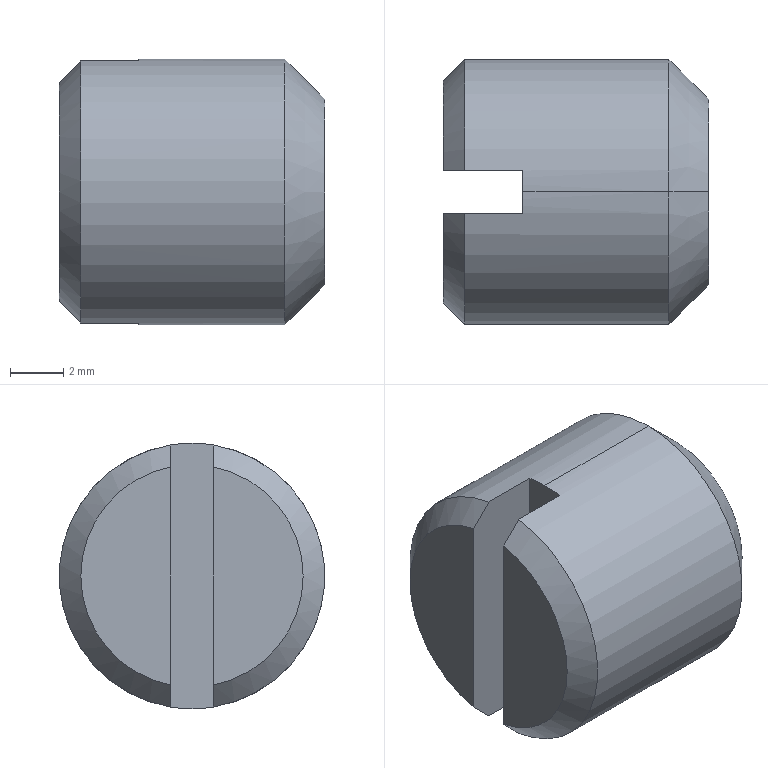Part | SolidWorks | features Cut 1, LPattern 1, RevCut 1, Revolution 1 | 1 solid | 12 faces | box 10 x 10 x 10 mm | volume 697.059 mm3 | plane 6 | cone 4 | cylinder 2 | commonest cylinder face diameters 10 x2
STEP:
#1=CARTESIAN_POINT('',(8.5,0.,5.));
#2=VERTEX_POINT('',#1);
#3=CARTESIAN_POINT('',(8.5,0.,-5.));
#4=VERTEX_POINT('',#3);
#5=CARTESIAN_POINT('',(8.5,0.,0.));
#6=DIRECTION('',(-1.,0.,0.));
#7=DIRECTION('',(0.,0.,1.));
#8=AXIS2_PLACEMENT_3D('',#5,#6,#7);
#9=CIRCLE('',#8,5.);
#10=EDGE_CURVE('',#2,#4,#9,.T.);
#11=ORIENTED_EDGE('',*,*,#10,.T.);
#12=CARTESIAN_POINT('',(3.,0.,-5.));
#13=VERTEX_POINT('',#12);
#14=CARTESIAN_POINT('',(-10.745,0.,-5.));
#15=DIRECTION('',(-1.,0.,0.));
#16=VECTOR('',#15,1000.);
#17=LINE('',#14,#16);
#18=EDGE_CURVE('',#4,#13,#17,.T.);
#19=ORIENTED_EDGE('',*,*,#18,.T.);
#20=CARTESIAN_POINT('',(3.,0.8,-4.936));
#21=VERTEX_POINT('',#20);
#22=CARTESIAN_POINT('',(3.,0.,0.));
#23=DIRECTION('',(1.,0.,0.));
#24=DIRECTION('',(0.,0.,-1.));
#25=AXIS2_PLACEMENT_3D('',#22,#23,#24);
#26=CIRCLE('',#25,5.);
#27=EDGE_CURVE('',#13,#21,#26,.T.);
#28=ORIENTED_EDGE('',*,*,#27,.T.);
#29=CARTESIAN_POINT('',(0.812,0.8,-4.936));
#30=VERTEX_POINT('',#29);
#31=CARTESIAN_POINT('',(-10.745,0.8,-4.936));
#32=DIRECTION('',(-1.,0.,0.));
#33=VECTOR('',#32,1000.);
#34=LINE('',#31,#33);
#35=EDGE_CURVE('',#21,#30,#34,.T.);
#36=ORIENTED_EDGE('',*,*,#35,.T.);
#37=CARTESIAN_POINT('',(0.812,0.8,4.936));
#38=VERTEX_POINT('',#37);
#39=CARTESIAN_POINT('',(0.812,0.,0.));
#40=DIRECTION('',(-1.,0.,0.));
#41=DIRECTION('',(0.,0.,1.));
#42=AXIS2_PLACEMENT_3D('',#39,#40,#41);
#43=CIRCLE('',#42,5.);
#44=EDGE_CURVE('',#38,#30,#43,.T.);
#45=ORIENTED_EDGE('',*,*,#44,.F.);
#46=CARTESIAN_POINT('',(3.,0.8,4.936));
#47=VERTEX_POINT('',#46);
#48=CARTESIAN_POINT('',(-10.745,0.8,4.936));
#49=DIRECTION('',(1.,0.,0.));
#50=VECTOR('',#49,1000.);
#51=LINE('',#48,#50);
#52=EDGE_CURVE('',#38,#47,#51,.T.);
#53=ORIENTED_EDGE('',*,*,#52,.T.);
#54=CARTESIAN_POINT('',(3.,0.,5.));
#55=VERTEX_POINT('',#54);
#56=CARTESIAN_POINT('',(3.,0.,0.));
#57=DIRECTION('',(1.,0.,0.));
#58=DIRECTION('',(0.,0.,-1.));
#59=AXIS2_PLACEMENT_3D('',#56,#57,#58);
#60=CIRCLE('',#59,5.);
#61=EDGE_CURVE('',#47,#55,#60,.T.);
#62=ORIENTED_EDGE('',*,*,#61,.T.);
#63=CARTESIAN_POINT('',(-10.745,0.,5.));
#64=DIRECTION('',(-1.,0.,0.));
#65=VECTOR('',#64,1000.);
#66=LINE('',#63,#65);
#67=EDGE_CURVE('',#2,#55,#66,.T.);
#68=ORIENTED_EDGE('',*,*,#67,.F.);
#69=EDGE_LOOP('',(#11,#19,#28,#36,#45,#53,#62,#68));
#70=FACE_OUTER_BOUND('',#69,.T.);
#71=CARTESIAN_POINT('',(-10.745,0.,0.));
#72=DIRECTION('',(-1.,0.,0.));
#73=DIRECTION('',(0.,0.,1.));
#74=AXIS2_PLACEMENT_3D('',#71,#72,#73);
#75=CYLINDRICAL_SURFACE('',#74,5.);
#76=ADVANCED_FACE('',(#70),#75,.T.);
#77=CARTESIAN_POINT('',(10.,0.,3.5));
#78=VERTEX_POINT('',#77);
#79=CARTESIAN_POINT('',(10.,0.,-3.5));
#80=VERTEX_POINT('',#79);
#81=CARTESIAN_POINT('',(10.,0.,0.));
#82=DIRECTION('',(-1.,0.,0.));
#83=DIRECTION('',(0.,0.,1.));
#84=AXIS2_PLACEMENT_3D('',#81,#82,#83);
#85=CIRCLE('',#84,3.5);
#86=EDGE_CURVE('',#78,#80,#85,.T.);
#87=ORIENTED_EDGE('',*,*,#86,.T.);
#88=CARTESIAN_POINT('',(10.,0.,-3.5));
#89=DIRECTION('',(-0.7071,0.,-0.7071));
#90=VECTOR('',#89,1000.);
#91=LINE('',#88,#90);
#92=EDGE_CURVE('',#80,#4,#91,.T.);
#93=ORIENTED_EDGE('',*,*,#92,.T.);
#94=ORIENTED_EDGE('',*,*,#10,.F.);
#95=CARTESIAN_POINT('',(10.,0.,3.5));
#96=DIRECTION('',(-0.7071,0.,0.7071));
#97=VECTOR('',#96,1000.);
#98=LINE('',#95,#97);
#99=EDGE_CURVE('',#78,#2,#98,.T.);
#100=ORIENTED_EDGE('',*,*,#99,.F.);
#101=EDGE_LOOP('',(#87,#93,#94,#100));
#102=FACE_OUTER_BOUND('',#101,.T.);
#103=CARTESIAN_POINT('',(10.,0.,0.));
#104=DIRECTION('',(-1.,0.,0.));
#105=DIRECTION('',(0.,0.,1.));
#106=AXIS2_PLACEMENT_3D('',#103,#104,#105);
#107=CONICAL_SURFACE('',#106,3.5,0.7854);
#108=ADVANCED_FACE('',(#102),#107,.T.);
#109=CARTESIAN_POINT('',(0.,0.8,4.111));
#110=VERTEX_POINT('',#109);
#111=CARTESIAN_POINT('',(0.,0.8,-4.111));
#112=VERTEX_POINT('',#111);
#113=CARTESIAN_POINT('',(0.,0.,0.));
#114=DIRECTION('',(-1.,0.,0.));
#115=DIRECTION('',(0.,0.,1.));
#116=AXIS2_PLACEMENT_3D('',#113,#114,#115);
#117=CIRCLE('',#116,4.188);
#118=EDGE_CURVE('',#110,#112,#117,.T.);
#119=ORIENTED_EDGE('',*,*,#118,.T.);
#120=CARTESIAN_POINT('',(0.,0.8,-5.));
#121=DIRECTION('',(0.,0.,1.));
#122=VECTOR('',#121,1000.);
#123=LINE('',#120,#122);
#124=EDGE_CURVE('',#112,#110,#123,.T.);
#125=ORIENTED_EDGE('',*,*,#124,.T.);
#126=EDGE_LOOP('',(#119,#125));
#127=FACE_OUTER_BOUND('',#126,.T.);
#128=CARTESIAN_POINT('',(0.,4.188,0.));
#129=DIRECTION('',(1.,0.,0.));
#130=DIRECTION('',(0.,0.,-1.));
#131=AXIS2_PLACEMENT_3D('',#128,#129,#130);
#132=PLANE('',#131);
#133=ADVANCED_FACE('',(#127),#132,.F.);
#134=ORIENTED_EDGE('',*,*,#44,.T.);
#135=CARTESIAN_POINT('',(0.812,0.8,-4.936));
#136=CARTESIAN_POINT('',(0.541,0.8,-4.661));
#137=CARTESIAN_POINT('',(0.2702,0.8,-4.386));
#138=CARTESIAN_POINT('',(0.,0.8,-4.111));
#139=B_SPLINE_CURVE_WITH_KNOTS('',3,(#135,#136,#137,#138),.UNSPECIFIED.,.F.,.F.,(4,4),(0.008538,0.009696),.UNSPECIFIED.);
#140=EDGE_CURVE('',#30,#112,#139,.T.);
#141=ORIENTED_EDGE('',*,*,#140,.T.);
#142=ORIENTED_EDGE('',*,*,#118,.F.);
#143=CARTESIAN_POINT('',(0.,0.8,4.111));
#144=CARTESIAN_POINT('',(0.2702,0.8,4.386));
#145=CARTESIAN_POINT('',(0.541,0.8,4.661));
#146=CARTESIAN_POINT('',(0.812,0.8,4.936));
#147=B_SPLINE_CURVE_WITH_KNOTS('',3,(#143,#144,#145,#146),.UNSPECIFIED.,.F.,.F.,(4,4),(0.0205,0.02167),.UNSPECIFIED.);
#148=EDGE_CURVE('',#110,#38,#147,.T.);
#149=ORIENTED_EDGE('',*,*,#148,.T.);
#150=EDGE_LOOP('',(#134,#141,#142,#149));
#151=FACE_OUTER_BOUND('',#150,.T.);
#152=CARTESIAN_POINT('',(0.812,0.,0.));
#153=DIRECTION('',(1.,0.,0.));
#154=DIRECTION('',(0.,0.,-1.));
#155=AXIS2_PLACEMENT_3D('',#152,#153,#154);
#156=CONICAL_SURFACE('',#155,5.,0.7854);
#157=ADVANCED_FACE('',(#151),#156,.T.);
#158=CARTESIAN_POINT('',(0.,-0.8,-4.111));
#159=VERTEX_POINT('',#158);
#160=CARTESIAN_POINT('',(0.,-0.8,4.111));
#161=VERTEX_POINT('',#160);
#162=CARTESIAN_POINT('',(0.,0.,0.));
#163=DIRECTION('',(-1.,0.,0.));
#164=DIRECTION('',(0.,0.,1.));
#165=AXIS2_PLACEMENT_3D('',#162,#163,#164);
#166=CIRCLE('',#165,4.188);
#167=EDGE_CURVE('',#159,#161,#166,.T.);
#168=ORIENTED_EDGE('',*,*,#167,.T.);
#169=CARTESIAN_POINT('',(0.,-0.8,-5.));
#170=DIRECTION('',(0.,0.,1.));
#171=VECTOR('',#170,1000.);
#172=LINE('',#169,#171);
#173=EDGE_CURVE('',#159,#161,#172,.T.);
#174=ORIENTED_EDGE('',*,*,#173,.F.);
#175=EDGE_LOOP('',(#168,#174));
#176=FACE_OUTER_BOUND('',#175,.T.);
#177=CARTESIAN_POINT('',(0.,4.188,0.));
#178=DIRECTION('',(1.,0.,0.));
#179=DIRECTION('',(0.,0.,-1.));
#180=AXIS2_PLACEMENT_3D('',#177,#178,#179);
#181=PLANE('',#180);
#182=ADVANCED_FACE('',(#176),#181,.F.);
#183=ORIENTED_EDGE('',*,*,#86,.F.);
#184=CARTESIAN_POINT('',(10.,0.,0.));
#185=DIRECTION('',(-1.,0.,0.));
#186=DIRECTION('',(0.,0.,1.));
#187=AXIS2_PLACEMENT_3D('',#184,#185,#186);
#188=CIRCLE('',#187,3.5);
#189=EDGE_CURVE('',#80,#78,#188,.T.);
#190=ORIENTED_EDGE('',*,*,#189,.F.);
#191=EDGE_LOOP('',(#183,#190));
#192=FACE_OUTER_BOUND('',#191,.T.);
#193=CARTESIAN_POINT('',(10.,0.,0.));
#194=DIRECTION('',(-1.,0.,0.));
#195=DIRECTION('',(0.,0.,1.));
#196=AXIS2_PLACEMENT_3D('',#193,#194,#195);
#197=PLANE('',#196);
#198=ADVANCED_FACE('',(#192),#197,.F.);
#199=ORIENTED_EDGE('',*,*,#92,.F.);
#200=ORIENTED_EDGE('',*,*,#189,.T.);
#201=ORIENTED_EDGE('',*,*,#99,.T.);
#202=CARTESIAN_POINT('',(8.5,0.,0.));
#203=DIRECTION('',(-1.,0.,0.));
#204=DIRECTION('',(0.,0.,1.));
#205=AXIS2_PLACEMENT_3D('',#202,#203,#204);
#206=CIRCLE('',#205,5.);
#207=EDGE_CURVE('',#4,#2,#206,.T.);
#208=ORIENTED_EDGE('',*,*,#207,.F.);
#209=EDGE_LOOP('',(#199,#200,#201,#208));
#210=FACE_OUTER_BOUND('',#209,.T.);
#211=CARTESIAN_POINT('',(10.,0.,0.));
#212=DIRECTION('',(-1.,0.,0.));
#213=DIRECTION('',(0.,0.,1.));
#214=AXIS2_PLACEMENT_3D('',#211,#212,#213);
#215=CONICAL_SURFACE('',#214,3.5,0.7854);
#216=ADVANCED_FACE('',(#210),#215,.T.);
#217=ORIENTED_EDGE('',*,*,#18,.F.);
#218=ORIENTED_EDGE('',*,*,#207,.T.);
#219=ORIENTED_EDGE('',*,*,#67,.T.);
#220=CARTESIAN_POINT('',(3.,-0.8,4.936));
#221=VERTEX_POINT('',#220);
#222=CARTESIAN_POINT('',(3.,0.,0.));
#223=DIRECTION('',(1.,0.,0.));
#224=DIRECTION('',(0.,0.,-1.));
#225=AXIS2_PLACEMENT_3D('',#222,#223,#224);
#226=CIRCLE('',#225,5.);
#227=EDGE_CURVE('',#55,#221,#226,.T.);
#228=ORIENTED_EDGE('',*,*,#227,.T.);
#229=CARTESIAN_POINT('',(0.812,-0.8,4.936));
#230=VERTEX_POINT('',#229);
#231=CARTESIAN_POINT('',(-10.745,-0.8,4.936));
#232=DIRECTION('',(-1.,0.,0.));
#233=VECTOR('',#232,1000.);
#234=LINE('',#231,#233);
#235=EDGE_CURVE('',#221,#230,#234,.T.);
#236=ORIENTED_EDGE('',*,*,#235,.T.);
#237=CARTESIAN_POINT('',(0.812,-0.8,-4.936));
#238=VERTEX_POINT('',#237);
#239=CARTESIAN_POINT('',(0.812,0.,0.));
#240=DIRECTION('',(-1.,0.,0.));
#241=DIRECTION('',(0.,0.,1.));
#242=AXIS2_PLACEMENT_3D('',#239,#240,#241);
#243=CIRCLE('',#242,5.);
#244=EDGE_CURVE('',#238,#230,#243,.T.);
#245=ORIENTED_EDGE('',*,*,#244,.F.);
#246=CARTESIAN_POINT('',(3.,-0.8,-4.936));
#247=VERTEX_POINT('',#246);
#248=CARTESIAN_POINT('',(-10.745,-0.8,-4.936));
#249=DIRECTION('',(1.,0.,0.));
#250=VECTOR('',#249,1000.);
#251=LINE('',#248,#250);
#252=EDGE_CURVE('',#238,#247,#251,.T.);
#253=ORIENTED_EDGE('',*,*,#252,.T.);
#254=CARTESIAN_POINT('',(3.,0.,0.));
#255=DIRECTION('',(1.,0.,0.));
#256=DIRECTION('',(0.,0.,-1.));
#257=AXIS2_PLACEMENT_3D('',#254,#255,#256);
#258=CIRCLE('',#257,5.);
#259=EDGE_CURVE('',#247,#13,#258,.T.);
#260=ORIENTED_EDGE('',*,*,#259,.T.);
#261=EDGE_LOOP('',(#217,#218,#219,#228,#236,#245,#253,#260));
#262=FACE_OUTER_BOUND('',#261,.T.);
#263=CARTESIAN_POINT('',(-10.745,0.,0.));
#264=DIRECTION('',(-1.,0.,0.));
#265=DIRECTION('',(0.,0.,1.));
#266=AXIS2_PLACEMENT_3D('',#263,#264,#265);
#267=CYLINDRICAL_SURFACE('',#266,5.);
#268=ADVANCED_FACE('',(#262),#267,.T.);
#269=ORIENTED_EDGE('',*,*,#244,.T.);
#270=CARTESIAN_POINT('',(0.812,-0.8,4.936));
#271=CARTESIAN_POINT('',(0.541,-0.8,4.661));
#272=CARTESIAN_POINT('',(0.2702,-0.8,4.386));
#273=CARTESIAN_POINT('',(0.,-0.8,4.111));
#274=B_SPLINE_CURVE_WITH_KNOTS('',3,(#270,#271,#272,#273),.UNSPECIFIED.,.F.,.F.,(4,4),(0.008538,0.009696),.UNSPECIFIED.);
#275=EDGE_CURVE('',#230,#161,#274,.T.);
#276=ORIENTED_EDGE('',*,*,#275,.T.);
#277=ORIENTED_EDGE('',*,*,#167,.F.);
#278=CARTESIAN_POINT('',(0.,-0.8,-4.111));
#279=CARTESIAN_POINT('',(0.2702,-0.8,-4.386));
#280=CARTESIAN_POINT('',(0.541,-0.8,-4.661));
#281=CARTESIAN_POINT('',(0.812,-0.8,-4.936));
#282=B_SPLINE_CURVE_WITH_KNOTS('',3,(#278,#279,#280,#281),.UNSPECIFIED.,.F.,.F.,(4,4),(0.0205,0.02167),.UNSPECIFIED.);
#283=EDGE_CURVE('',#159,#238,#282,.T.);
#284=ORIENTED_EDGE('',*,*,#283,.T.);
#285=EDGE_LOOP('',(#269,#276,#277,#284));
#286=FACE_OUTER_BOUND('',#285,.T.);
#287=CARTESIAN_POINT('',(0.812,0.,0.));
#288=DIRECTION('',(1.,0.,0.));
#289=DIRECTION('',(0.,0.,-1.));
#290=AXIS2_PLACEMENT_3D('',#287,#288,#289);
#291=CONICAL_SURFACE('',#290,5.,0.7854);
#292=ADVANCED_FACE('',(#286),#291,.T.);
#293=CARTESIAN_POINT('',(3.,0.8,-5.));
#294=DIRECTION('',(0.,0.,1.));
#295=VECTOR('',#294,1000.);
#296=LINE('',#293,#295);
#297=EDGE_CURVE('',#21,#47,#296,.T.);
#298=ORIENTED_EDGE('',*,*,#297,.F.);
#299=ORIENTED_EDGE('',*,*,#27,.F.);
#300=ORIENTED_EDGE('',*,*,#259,.F.);
#301=CARTESIAN_POINT('',(3.,-0.8,-5.));
#302=DIRECTION('',(0.,0.,1.));
#303=VECTOR('',#302,1000.);
#304=LINE('',#301,#303);
#305=EDGE_CURVE('',#247,#221,#304,.T.);
#306=ORIENTED_EDGE('',*,*,#305,.T.);
#307=ORIENTED_EDGE('',*,*,#227,.F.);
#308=ORIENTED_EDGE('',*,*,#61,.F.);
#309=EDGE_LOOP('',(#298,#299,#300,#306,#307,#308));
#310=FACE_OUTER_BOUND('',#309,.T.);
#311=CARTESIAN_POINT('',(3.,0.8,-5.));
#312=DIRECTION('',(1.,0.,0.));
#313=DIRECTION('',(0.,0.,-1.));
#314=AXIS2_PLACEMENT_3D('',#311,#312,#313);
#315=PLANE('',#314);
#316=ADVANCED_FACE('',(#310),#315,.F.);
#317=ORIENTED_EDGE('',*,*,#297,.T.);
#318=ORIENTED_EDGE('',*,*,#52,.F.);
#319=ORIENTED_EDGE('',*,*,#148,.F.);
#320=ORIENTED_EDGE('',*,*,#124,.F.);
#321=ORIENTED_EDGE('',*,*,#140,.F.);
#322=ORIENTED_EDGE('',*,*,#35,.F.);
#323=EDGE_LOOP('',(#317,#318,#319,#320,#321,#322));
#324=FACE_OUTER_BOUND('',#323,.T.);
#325=CARTESIAN_POINT('',(0.,0.8,-5.));
#326=DIRECTION('',(0.,1.,0.));
#327=DIRECTION('',(0.,0.,1.));
#328=AXIS2_PLACEMENT_3D('',#325,#326,#327);
#329=PLANE('',#328);
#330=ADVANCED_FACE('',(#324),#329,.F.);
#331=ORIENTED_EDGE('',*,*,#305,.F.);
#332=ORIENTED_EDGE('',*,*,#252,.F.);
#333=ORIENTED_EDGE('',*,*,#283,.F.);
#334=ORIENTED_EDGE('',*,*,#173,.T.);
#335=ORIENTED_EDGE('',*,*,#275,.F.);
#336=ORIENTED_EDGE('',*,*,#235,.F.);
#337=EDGE_LOOP('',(#331,#332,#333,#334,#335,#336));
#338=FACE_OUTER_BOUND('',#337,.T.);
#339=CARTESIAN_POINT('',(0.,-0.8,-5.));
#340=DIRECTION('',(0.,-1.,0.));
#341=DIRECTION('',(0.,0.,-1.));
#342=AXIS2_PLACEMENT_3D('',#339,#340,#341);
#343=PLANE('',#342);
#344=ADVANCED_FACE('',(#338),#343,.F.);
#345=CLOSED_SHELL('',(#76,#108,#133,#157,#182,#198,#216,#268,#292,#316,#330,#344));
#346=MANIFOLD_SOLID_BREP('',#345);
#347=CARTESIAN_POINT('',(0.,0.,0.));
#348=DIRECTION('',(0.,0.,1.));
#349=DIRECTION('',(1.,0.,0.));
#350=AXIS2_PLACEMENT_3D('',#347,#348,#349);
#351=(LENGTH_UNIT()NAMED_UNIT(*)SI_UNIT(.MILLI.,.METRE.));
#352=UNCERTAINTY_MEASURE_WITH_UNIT(LENGTH_MEASURE(0.00001),#351,'','');
#353=(NAMED_UNIT(*)PLANE_ANGLE_UNIT()SI_UNIT($,.RADIAN.));
#354=(NAMED_UNIT(*)SI_UNIT($,.STERADIAN.)SOLID_ANGLE_UNIT());
#355=(GEOMETRIC_REPRESENTATION_CONTEXT(3)GLOBAL_UNCERTAINTY_ASSIGNED_CONTEXT((#352))GLOBAL_UNIT_ASSIGNED_CONTEXT((#351,#353,#354))REPRESENTATION_CONTEXT('',''));
#356=ADVANCED_BREP_SHAPE_REPRESENTATION('',(#346,#350),#355);